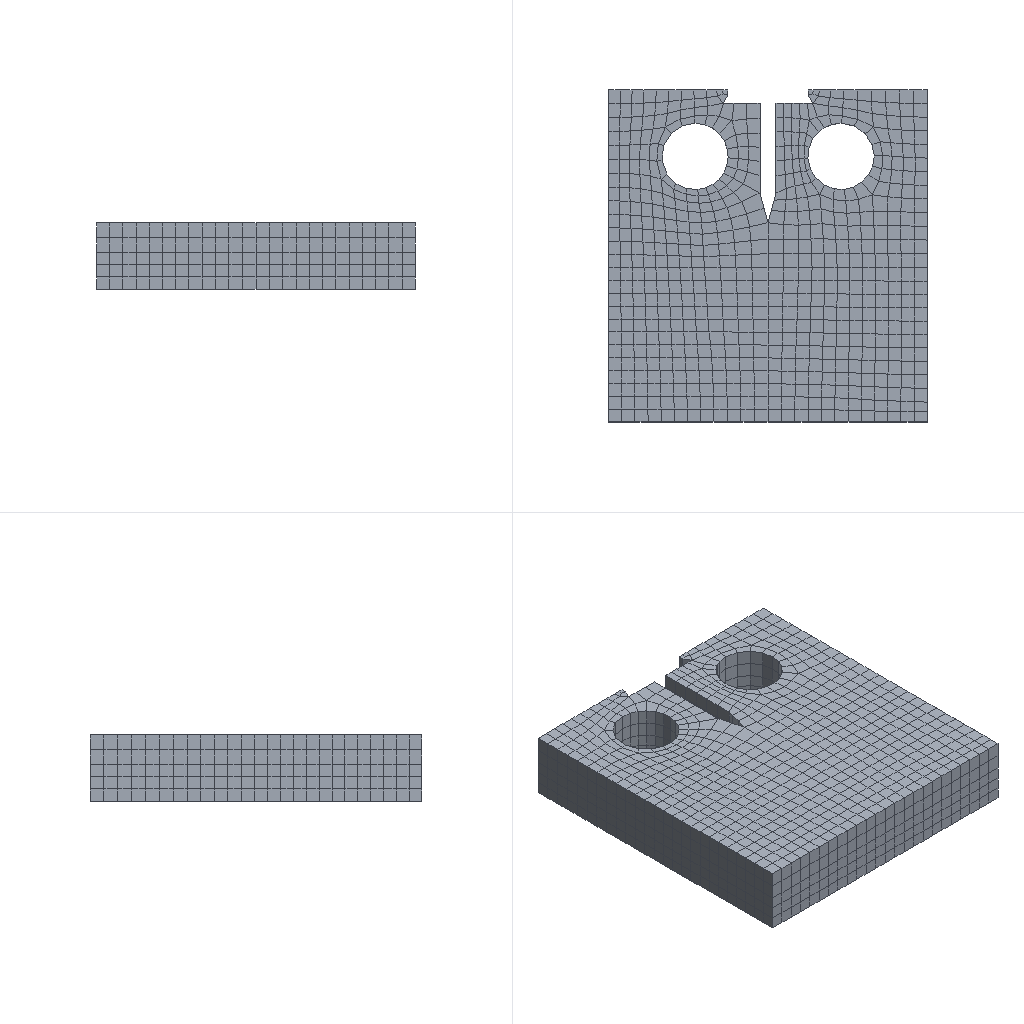Simulation study | abaqus
Set-up summary:
category,name,step,type,value,unit,region
solver,abaqus,,Abaqus/CAE 2024
units,mm-N-s-tonne (MPa),,inferred,E=227000 density=8.14e-09
analysis,Step-1,,static,nlgeom=True; time_period=10
mesh,nodes,,,4124
mesh,elements,,,3030
element_type,C3D8R,,,3030
material,Material-1,,E,227000
material,Material-1,,nu,0.35
material,Material-1,,density,8.14e-09
material,Material-1,,conductivity,0.0125
material,Material-1,,specific_heat,476300
material,Material-1,,cte,8.6152e-06
material,Material-1,,behaviors,conductivity; damage initiation; damage evolution; expansion; specific heat
section,Material-1,,solid section,,,Set-1
bc,BC-1,initial,encastre,[dofs=ENCASTRE],,_PickedSet51
bc,BC-2,Step-1,displacement,8 [dofs=x],,_PickedSet52
bc,BC-2,Step-1,fixed,"[dofs=rx,ry,z n=3]",,_PickedSet52
constraint,coupling,,,2
Abaqus input file, long lists of numbers shortened:
*Heading
** Job name: deck Model name: Model-1
** Generated by: Abaqus/CAE 2024
*Preprint, echo=NO, model=NO, history=NO, contact=NO
**
** PARTS
**
*Part, name=Part-1
*Node
      1,           0., -0.1986,         12.5
      2,           0.,  -29.23,         12.5
** (4120 more lines like these left out)
*Element, type=C3D8R
   1,   65,  201,   23,    1,  752,  888,  710,  688
   2,  201,  202,   24,   23,  888,  889,  711,  710
** (3028 more lines like these left out)
*Nset, nset=Set-1, generate
    1,  4122,     1
*Elset, elset=Set-1, generate
    1,  3030,     1
** Section: Section-1
*Solid Section, elset=Set-1, material=Material-1
,
*End Part
**
**
** ASSEMBLY
**
*Assembly, name=Assembly
**
*Instance, name=Part-1-2, part=Part-1
*End Instance
**
*Node
      1,       -13.75,   20.77,         6.25
*Node
      2,        13.75,   20.77,         6.25
*Nset, nset=Set-3, instance=Part-1-2, generate
    1,  4122,     1
*Elset, elset=Set-3, instance=Part-1-2, generate
    1,  3030,     1
*Nset, nset=Set-4, instance=Part-1-2, generate
    1,  4122,     1
*Elset, elset=Set-4, instance=Part-1-2, generate
    1,  3030,     1
*Nset, nset=Set-5, instance=Part-1-2, generate
    1,  4122,     1
*Elset, elset=Set-5, instance=Part-1-2, generate
    1,  3030,     1
*Nset, nset=Set-6, instance=Part-1-2, generate
    1,  4122,     1
*Elset, elset=Set-6, instance=Part-1-2, generate
    1,  3030,     1
*Nset, nset=Set-7, instance=Part-1-2
    2,    4,   15,   34,   35,   36,   37,   38,   39,   40,   41,   42,   43,   44,  141,  142
  143,  144,  145,  146,  147,  148,  149,  150,  151,  689,  691,  702,  721,  722,  723,  724
** (8 more lines like these left out)
*Elset, elset=Set-7, instance=Part-1-2
   12,   24,   36,   48,   60,   72,   84,   96,  108,  120,  132,  144,  312,  324,  336,  348
  360,  372,  384,  396,  408,  420,  432,  444,  618,  630,  642,  654,  666,  678,  690,  702
** (6 more lines like these left out)
*Nset, nset=Set-8, instance=Part-1-2
    1,    2,    4,    5,    6,    9,   14,   16,   17,   19,   21,   22, 3439, 3441, 3443, 3444
 3451, 3452, 3454, 3455, 3456, 3457
*Nset, nset=Set-9, instance=Part-1-2
    1,    2,    6,    7,    8,    9,   10,   11,   12,   13,   16,   17,   19,   20,   21,   22
 3441, 3442, 3443, 3444, 3445, 3447, 3448, 3451, 3452, 3453, 3454, 3455, 3456, 3457
*Nset, nset=Set-10, instance=Part-1-2, generate
    1,  4122,     1
*Elset, elset=Set-10, instance=Part-1-2, generate
    1,  3030,     1
*Nset, nset=Set-11, instance=Part-1-2
    2,    4,   15,   34,   35,   36,   37,   38,   39,   40,   41,   42,   43,   44,  141,  142
  143,  144,  145,  146,  147,  148,  149,  150,  151,  689,  691,  702,  721,  722,  723,  724
** (8 more lines like these left out)
*Elset, elset=Set-11, instance=Part-1-2
   12,   24,   36,   48,   60,   72,   84,   96,  108,  120,  132,  144,  312,  324,  336,  348
  360,  372,  384,  396,  408,  420,  432,  444,  618,  630,  642,  654,  666,  678,  690,  702
** (6 more lines like these left out)
*Nset, nset=Set-12, instance=Part-1-2
    3,    4,    5,   11,   45,   46,   47,   48,   49,   50,   51,   52,   53,   54,   66,   67
   68,   69,   70,   71,   72,   73,   74,   75,   76,   77,  690,  691,  692,  698,  732,  733
** (8 more lines like these left out)
*Elset, elset=Set-12, instance=Part-1-2
  133,  134,  135,  136,  137,  138,  139,  140,  141,  142,  143,  144,  236,  240,  244,  248
  252,  253,  254,  255,  273,  277,  278,  279,  280,  739,  740,  741,  742,  743,  744,  745
** (6 more lines like these left out)
*Nset, nset=Set-13, instance=Part-1-2
    5,    6,    7,    8,    9,   10,   12,   13,   16,   17,   18,   19,   20,   21,   22, 3441
 3442, 3443, 3444, 3445, 3447, 3448, 3451, 3452, 3453, 3454, 3455, 3456, 3457
*Nset, nset=Set-14, instance=Part-1-2, generate
 3436,  4122,     1
*Elset, elset=Set-14, instance=Part-1-2, generate
 2425,  3030,     1
*Nset, nset=Set-15, instance=Part-1-2
    2,    4,   15,   34,   35,   36,   37,   38,   39,   40,   41,   42,   43,   44,  141,  142
  143,  144,  145,  146,  147,  148,  149,  150,  151,  689,  691,  702,  721,  722,  723,  724
** (8 more lines like these left out)
*Elset, elset=Set-15, instance=Part-1-2
   12,   24,   36,   48,   60,   72,   84,   96,  108,  120,  132,  144,  312,  324,  336,  348
  360,  372,  384,  396,  408,  420,  432,  444,  618,  630,  642,  654,  666,  678,  690,  702
** (6 more lines like these left out)
*Nset, nset=Set-16, instance=Part-1-2
    2,    4,   15,   34,   35,   36,   37,   38,   39,   40,   41,   42,   43,   44,  141,  142
  143,  144,  145,  146,  147,  148,  149,  150,  151,  689,  691,  702,  721,  722,  723,  724
** (8 more lines like these left out)
*Elset, elset=Set-16, instance=Part-1-2
   12,   24,   36,   48,   60,   72,   84,   96,  108,  120,  132,  144,  312,  324,  336,  348
  360,  372,  384,  396,  408,  420,  432,  444,  618,  630,  642,  654,  666,  678,  690,  702
** (6 more lines like these left out)
*Nset, nset=Set-17, instance=Part-1-2
    2,    4,   15,   34,   35,   36,   37,   38,   39,   40,   41,   42,   43,   44,  141,  142
  143,  144,  145,  146,  147,  148,  149,  150,  151,  689,  691,  702,  721,  722,  723,  724
** (8 more lines like these left out)
*Elset, elset=Set-17, instance=Part-1-2
   12,   24,   36,   48,   60,   72,   84,   96,  108,  120,  132,  144,  312,  324,  336,  348
  360,  372,  384,  396,  408,  420,  432,  444,  618,  630,  642,  654,  666,  678,  690,  702
** (6 more lines like these left out)
*Nset, nset=Set-18, instance=Part-1-2
    2,    4,   15,   34,   35,   36,   37,   38,   39,   40,   41,   42,   43,   44,  141,  142
  143,  144,  145,  146,  147,  148,  149,  150,  151,  689,  691,  702,  721,  722,  723,  724
** (8 more lines like these left out)
*Elset, elset=Set-18, instance=Part-1-2
   12,   24,   36,   48,   60,   72,   84,   96,  108,  120,  132,  144,  312,  324,  336,  348
  360,  372,  384,  396,  408,  420,  432,  444,  618,  630,  642,  654,  666,  678,  690,  702
** (6 more lines like these left out)
*Nset, nset=Set-19, instance=Part-1-2
 1,
*Nset, nset=Set-20, instance=Part-1-2, generate
    1,  4122,     1
*Elset, elset=Set-20, instance=Part-1-2, generate
    1,  3030,     1
*Nset, nset=Set-21, instance=Part-1-2, generate
    1,  4122,     1
*Elset, elset=Set-21, instance=Part-1-2, generate
    1,  3030,     1
*Nset, nset=Set-22, instance=Part-1-2
   16,  152,  153,  154,  155,  156,  157,  158,  159,  160,  161,  162,  163,  164,  165,  166
  167,  168,  169,  170,  703,  839,  840,  841,  842,  843,  844,  845,  846,  847,  848,  849
** (6 more lines like these left out)
*Elset, elset=Set-22, instance=Part-1-2
  448,  452,  463,  464,  465,  466,  488,  489,  490,  491,  492,  506,  531,  532,  533,  534
  575,  583,  591,  599, 1054, 1058, 1069, 1070, 1071, 1072, 1094, 1095, 1096, 1097, 1098, 1112
** (5 more lines like these left out)
*Nset, nset=Set-23, instance=Part-1-2
   10,  100,  101,  102,  103,  104,  105,  106,  107,  108,  109,  110,  111,  112,  113,  114
  115,  116,  117,  118,  697,  787,  788,  789,  790,  791,  792,  793,  794,  795,  796,  797
** (6 more lines like these left out)
*Elset, elset=Set-23, instance=Part-1-2
  165,  166,  167,  168,  169,  170,  198,  199,  200,  213,  217,  221,  222,  265,  266,  267
  268,  269,  296,  297,  771,  772,  773,  774,  775,  776,  804,  805,  806,  819,  823,  827
** (5 more lines like these left out)
*Nset, nset=Set-24, instance=Part-1-2
 10,
*Nset, nset=Set-25, instance=Part-1-2
 16,
*Nset, nset=Set-26, instance=Part-1-2
    2,    4,   15,   34,   35,   36,   37,   38,   39,   40,   41,   42,   43,   44,  141,  142
  143,  144,  145,  146,  147,  148,  149,  150,  151,  689,  691,  702,  721,  722,  723,  724
** (8 more lines like these left out)
*Elset, elset=Set-26, instance=Part-1-2
   12,   24,   36,   48,   60,   72,   84,   96,  108,  120,  132,  144,  312,  324,  336,  348
  360,  372,  384,  396,  408,  420,  432,  444,  618,  630,  642,  654,  666,  678,  690,  702
** (6 more lines like these left out)
*Nset, nset=m_Set-32
 1,
*Nset, nset=_PickedSet34, internal, instance=Part-1-2, generate
    1,  4122,     1
*Elset, elset=_PickedSet34, internal, instance=Part-1-2, generate
    1,  3030,     1
*Nset, nset=_PickedSet50, internal
 2,
*Nset, nset=_PickedSet51, internal
 1,
*Nset, nset=_PickedSet52, internal
 2,
*Elset, elset=_Surf-1_S1, internal, instance=Part-1-2
   1,   2,   3,   4,   5,   6,   7,   8,   9,  10,  11,  12,  13,  14,  15,  16
  17,  18,  19,  20,  21,  22,  23,  24,  25,  26,  27,  28,  29,  30,  31,  32
** (16 more lines like these left out)
*Elset, elset=_Surf-1_S6, internal, instance=Part-1-2
  213,  217,  445,  449,  575,  583,  591,  599,  819,  823, 1051, 1055, 1181, 1189, 1197, 1205
 1425, 1429, 1657, 1661, 1787, 1795, 1803, 1811, 2031, 2035, 2263, 2267, 2393, 2401, 2409, 2417
** (1 more lines like these left out)
*Elset, elset=_Surf-1_S4, internal, instance=Part-1-2
   12,   24,   36,   48,   60,   72,   84,   96,  108,  120,  132,  144,  165,  166,  167,  168
  169,  171,  175,  198,  199,  216,  220,  236,  240,  244,  248,  252,  265,  266,  267,  273
** (22 more lines like these left out)
*Elset, elset=_Surf-1_S5, internal, instance=Part-1-2
  145,  146,  147,  148,  149,  170,  172,  173,  174,  175,  200,  221,  222,  253,  254,  255
  268,  269,  278,  279,  280,  290,  291,  298,  300,  301,  302,  303,  304,  305,  306,  307
** (18 more lines like these left out)
*Elset, elset=_Surf-1_S3, internal, instance=Part-1-2
  133,  134,  135,  136,  137,  138,  139,  140,  141,  142,  143,  144,  185,  186,  187,  602
  603,  739,  740,  741,  742,  743,  744,  745,  746,  747,  748,  749,  750,  791,  792,  793
** (4 more lines like these left out)
*Elset, elset=_Surf-1_S2, internal, instance=Part-1-2, generate
 2425,  3030,     1
*Surface, type=ELEMENT, name=Surf-1
_Surf-1_S1, S1
_Surf-1_S6, S6
_Surf-1_S4, S4
_Surf-1_S2, S2
_Surf-1_S5, S5
_Surf-1_S3, S3
*Elset, elset=_Surf-2_S1, internal, instance=Part-1-2, generate
   1,  606,    1
*Elset, elset=_Surf-2_S4, internal, instance=Part-1-2
  165,  166,  167,  168,  169,  175,  198,  199,  265,  266,  267,  296,  297,  448,  452,  463
  464,  494,  496,  498,  500,  502,  506,  531,  532,  533,  771,  772,  773,  774,  775,  781
** (7 more lines like these left out)
*Elset, elset=_Surf-2_S5, internal, instance=Part-1-2
  145,  146,  147,  148,  149,  170,  200,  221,  222,  268,  269,  465,  466,  488,  489,  490
  491,  492,  503,  534,  751,  752,  753,  754,  755,  776,  806,  827,  828,  874,  875, 1071
** (5 more lines like these left out)
*Elset, elset=_Surf-2_S3, internal, instance=Part-1-2
  185,  186,  187,  602,  603,  791,  792,  793, 1208, 1209, 1397, 1398, 1399, 1814, 1815, 2003
 2004, 2005, 2420, 2421, 2609, 2610, 2611, 3026, 3027
*Elset, elset=_Surf-2_S6, internal, instance=Part-1-2
  213,  217,  575,  583,  591,  599,  819,  823, 1181, 1189, 1197, 1205, 1425, 1429, 1787, 1795
 1803, 1811, 2031, 2035, 2393, 2401, 2409, 2417, 2637, 2641, 2999, 3007, 3015, 3023
*Surface, type=ELEMENT, name=Surf-2
_Surf-2_S1, S1
_Surf-2_S4, S4
_Surf-2_S6, S6
_Surf-2_S5, S5
_Surf-2_S3, S3
*Elset, elset=__PickedSurf39_S4, internal, instance=Part-1-2
  448,  452,  463,  464,  506,  531,  532,  533, 1054, 1058, 1069, 1070, 1112, 1137, 1138, 1139
 1660, 1664, 1675, 1676, 1718, 1743, 1744, 1745, 2266, 2270, 2281, 2282, 2324, 2349, 2350, 2351
** (1 more lines like these left out)
*Elset, elset=__PickedSurf39_S5, internal, instance=Part-1-2
  465,  466,  488,  489,  490,  491,  492,  534, 1071, 1072, 1094, 1095, 1096, 1097, 1098, 1140
 1677, 1678, 1700, 1701, 1702, 1703, 1704, 1746, 2283, 2284, 2306, 2307, 2308, 2309, 2310, 2352
** (1 more lines like these left out)
*Elset, elset=__PickedSurf39_S6, internal, instance=Part-1-2
  575,  583,  591,  599, 1181, 1189, 1197, 1205, 1787, 1795, 1803, 1811, 2393, 2401, 2409, 2417
 2999, 3007, 3015, 3023
*Surface, type=ELEMENT, name=_PickedSurf39, internal
__PickedSurf39_S4, S4
__PickedSurf39_S5, S5
__PickedSurf39_S6, S6
*Elset, elset=__PickedSurf41_S4, internal, instance=Part-1-2
  165,  166,  167,  168,  169,  198,  199,  265,  266,  267,  296,  297,  771,  772,  773,  774
  775,  804,  805,  871,  872,  873,  902,  903, 1377, 1378, 1379, 1380, 1381, 1410, 1411, 1477
** (2 more lines like these left out)
*Elset, elset=__PickedSurf41_S5, internal, instance=Part-1-2
  170,  200,  221,  222,  268,  269,  776,  806,  827,  828,  874,  875, 1382, 1412, 1433, 1434
 1480, 1481, 1988, 2018, 2039, 2040, 2086, 2087, 2594, 2624, 2645, 2646, 2692, 2693
*Elset, elset=__PickedSurf41_S6, internal, instance=Part-1-2
  213,  217,  819,  823, 1425, 1429, 2031, 2035, 2637, 2641
*Surface, type=ELEMENT, name=_PickedSurf41, internal
__PickedSurf41_S4, S4
__PickedSurf41_S5, S5
__PickedSurf41_S6, S6
** Constraint: Constraint-1
*Coupling, constraint name=Constraint-1, ref node=m_Set-32, surface=_PickedSurf39
*Kinematic
** Constraint: Constraint-2
*Coupling, constraint name=Constraint-2, ref node=_PickedSet50, surface=_PickedSurf41
*Kinematic
*Enrichment, name=Crack-1, type=PROPAGATION CRACK, elset=_PickedSet34
*End Assembly
*Amplitude, name=Amp-1, definition=PERIODIC
3,             1.2,             0.1,             25.
            0.1,             25.,             0.2,             50.,             0.3,            100.
*Amplitude, name=Amp-2, definition=PERIODIC
3,             1.1,             0.1,             25.
            0.1,             25.,             0.2,             50.,             0.3,            100.
*Amplitude, name=Amp-3, definition=PERIODIC
1,             10.,             0.1,             20.
            20.,             20.
*Amplitude, name=Amp-4, definition=PERIODIC
2,             10.,             0.1,             20.
            0.1,             20.,             0.2,             50.
*Amplitude, name=Amp-5, definition=PERIODIC
2,             10.,             0.1,             20.
            0.1,             20.,             0.2,             50.
*Amplitude, name=Amp-6, definition=PERIODIC
1,             10.,             0.1,             10.
            0.1,             10.
*Amplitude, name=Amp-7, definition=PERIODIC
2,            110.,             0.1,              0.
             0.,              0.,             0.1,              1.
*Amplitude, name=Amp-8, definition=PERIODIC
1,             10.,              0.,              0.
             0.,             20.
*Amplitude, name=Amp-9
             0.,              0.,            0.25,             0.5,             0.5,            -0.5,            0.75,              1.
            0.9,             -1.,              1.,              0.
*Amplitude, name=Amp-10
             0.,              0.,              1.,              1.,              2.,             -1.,              3.,              1.
             4.,             -1.,              5.,              1.,              6.,             -1.,              7.,              1.
             8.,             -1.,              9.,              1.,             10.,             -1.
**
** MATERIALS
**
*Material, name=Material-1
*Conductivity
 0.0125, 20.
  0.014,100.
 0.0158,200.
 0.0175,300.
 0.0193,400.
  0.021,500.
 0.0225,600.
 0.0238,700.
  0.025,800.
*Damage Initiation, criterion=QUADS
235.,235.,235.
*Damage Evolution, type=DISPLACEMENT
5.,
*Density
 8.14e-09,
*Elastic
227000., 0.35,  20.
222000., 0.35, 100.
217000., 0.36, 200.
212000., 0.36, 300.
207000., 0.37, 400.
202000., 0.37, 500.
196000., 0.38, 600.
192000., 0.38, 650.
189000., 0.38, 700.
184000., 0.39, 750.
182000., 0.39, 800.
*Expansion, zero=25.
  8.6152e-06, 50.
 1.03376e-05,100.
 1.10482e-05,200.
 1.15461e-05,300.
 1.19375e-05,400.
 1.22776e-05,500.
  1.2553e-05,600.
 1.30705e-05,700.
  1.3804e-05,800.
*Specific Heat
476300.,  50.
478900., 100.
488000., 200.
506800., 300.
525000., 400.
533800., 500.
552100., 600.
596600., 700.
649700., 800.
690700., 900.
722900.,1000.
**
** BOUNDARY CONDITIONS
**
** Name: BC-1 Type: Symmetry/Antisymmetry/Encastre
*Boundary
_PickedSet51, ENCASTRE
** ----------------------------------------------------------------
**
** STEP: Step-1
**
*Step, name=Step-1, nlgeom=YES, inc=10000
*Static, stabilize=0.0002, allsdtol=0.05, continue=NO
0.01, 10., 1e-07, 0.1
**
** BOUNDARY CONDITIONS
**
** Name: BC-2 Type: Displacement/Rotation
*Boundary, amplitude=Amp-10
_PickedSet52, 1, 1, 8.
_PickedSet52, 3, 3
_PickedSet52, 4, 4
_PickedSet52, 5, 5
**
** CONTROLS
**
*Controls, reset
*Controls, parameters=time incrementation
, , , , , , , 10, , ,
**
** OUTPUT REQUESTS
**
*Restart, write, frequency=0
**
** FIELD OUTPUT: F-Output-1
**
*Output, field
*Node Output
CF, PHILSM, PSILSM, RF, U
*Element Output, directions=YES
LE, PE, PEEQ, PEMAG, S, SDEG, STATUSXFEM
*Contact Output
CDISP, CSTRESS
**
** HISTORY OUTPUT: H-Output-1
**
*Output, history, variable=PRESELECT
*End Step
Results summary:
result,odb.job_status,,,JOB_STATUS_EXITED_WITH_ERROR,"consistent, unstated (Abaqus has no unit system)"
result,steps[0].procedure,Step-1,,*STATIC,"consistent, unstated (Abaqus has no unit system)"
result,steps[0].time_period,Step-1,,0.06342,"consistent, unstated (Abaqus has no unit system)"
result,steps[0].n_frames,Step-1,,113,"consistent, unstated (Abaqus has no unit system)"
result,steps[0].last_frame.id,Step-1,,112,"consistent, unstated (Abaqus has no unit system)"
result,steps[0].last_frame.value,Step-1,,0.06342,"consistent, unstated (Abaqus has no unit system)"
result,steps[0].last_frame.description,Step-1,,Increment    112: Step Time =   6.3418E-02,"consistent, unstated (Abaqus has no unit system)"
result,steps[0].completed,Step-1,,True,"consistent, unstated (Abaqus has no unit system)"
result,steps[0].max_U_magnitude,Step-1,,0.8924,"consistent, unstated (Abaqus has no unit system)"
result,steps[0].max_S_mises,Step-1,,7235.09,"consistent, unstated (Abaqus has no unit system)"
result,steps[0].RF_sum[1],Step-1,,-5001.48,"consistent, unstated (Abaqus has no unit system)"
result,steps[0].RF_sum[2],Step-1,,1617.77,"consistent, unstated (Abaqus has no unit system)"
result,steps[0].RF_sum[3],Step-1,,-420.4,"consistent, unstated (Abaqus has no unit system)"